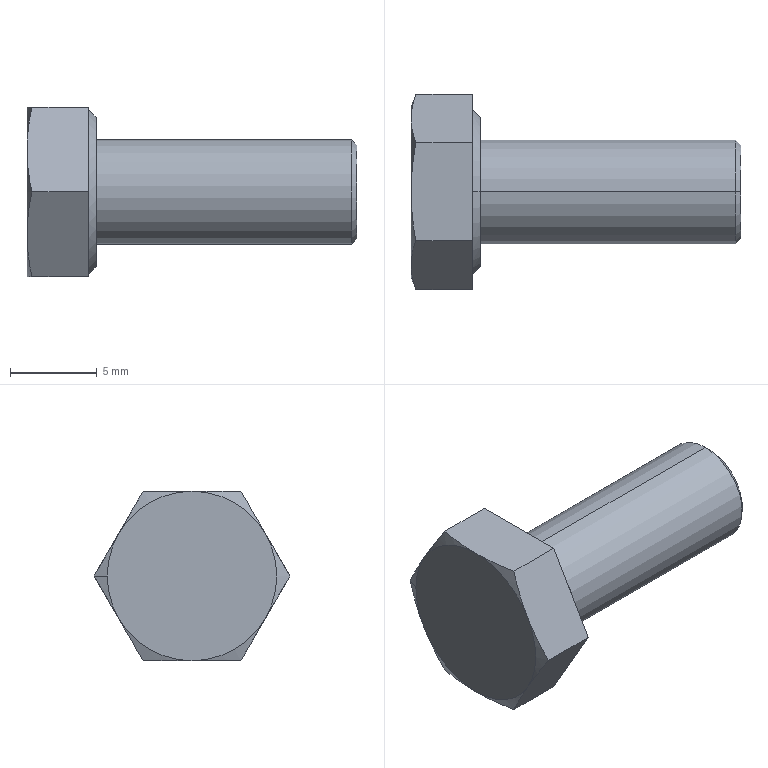Part | SolidWorks | features BaseBody 1, MoveFace 1, Scale 1 | 1 solid | 23 faces | box 18.975 x 11.258 x 9.75 mm | volume 741.836 mm3 | cone 11 | plane 10 | cylinder 2 | commonest cylinder face diameters 6 x2
STEP:
#1=CARTESIAN_POINT('',(18.675,0.,3.));
#2=VERTEX_POINT('',#1);
#3=CARTESIAN_POINT('',(18.675,0.,-3.));
#4=VERTEX_POINT('',#3);
#5=CARTESIAN_POINT('',(18.675,0.,0.));
#6=DIRECTION('',(-1.,0.,0.));
#7=DIRECTION('',(0.,0.,1.));
#8=AXIS2_PLACEMENT_3D('',#5,#6,#7);
#9=CIRCLE('',#8,3.);
#10=EDGE_CURVE('',#2,#4,#9,.T.);
#11=ORIENTED_EDGE('',*,*,#10,.T.);
#12=CARTESIAN_POINT('',(3.975,0.,-3.));
#13=VERTEX_POINT('',#12);
#14=CARTESIAN_POINT('',(33.975,0.,-3.));
#15=DIRECTION('',(-1.,0.,0.));
#16=VECTOR('',#15,1000.);
#17=LINE('',#14,#16);
#18=EDGE_CURVE('',#4,#13,#17,.T.);
#19=ORIENTED_EDGE('',*,*,#18,.T.);
#20=CARTESIAN_POINT('',(3.975,0.,3.));
#21=VERTEX_POINT('',#20);
#22=CARTESIAN_POINT('',(3.975,0.,0.));
#23=DIRECTION('',(1.,0.,0.));
#24=DIRECTION('',(0.,0.,1.));
#25=AXIS2_PLACEMENT_3D('',#22,#23,#24);
#26=CIRCLE('',#25,3.);
#27=EDGE_CURVE('',#13,#21,#26,.T.);
#28=ORIENTED_EDGE('',*,*,#27,.T.);
#29=CARTESIAN_POINT('',(33.975,0.,3.));
#30=DIRECTION('',(-1.,0.,0.));
#31=VECTOR('',#30,1000.);
#32=LINE('',#29,#31);
#33=EDGE_CURVE('',#2,#21,#32,.T.);
#34=ORIENTED_EDGE('',*,*,#33,.F.);
#35=EDGE_LOOP('',(#11,#19,#28,#34));
#36=FACE_OUTER_BOUND('',#35,.T.);
#37=CARTESIAN_POINT('',(33.975,0.,0.));
#38=DIRECTION('',(-1.,0.,0.));
#39=DIRECTION('',(0.,0.,1.));
#40=AXIS2_PLACEMENT_3D('',#37,#38,#39);
#41=CYLINDRICAL_SURFACE('',#40,3.);
#42=ADVANCED_FACE('',(#36),#41,.T.);
#43=CARTESIAN_POINT('',(18.975,0.,2.7));
#44=VERTEX_POINT('',#43);
#45=CARTESIAN_POINT('',(18.975,0.,-2.7));
#46=VERTEX_POINT('',#45);
#47=CARTESIAN_POINT('',(18.975,0.,0.));
#48=DIRECTION('',(-1.,0.,0.));
#49=DIRECTION('',(0.,0.,1.));
#50=AXIS2_PLACEMENT_3D('',#47,#48,#49);
#51=CIRCLE('',#50,2.7);
#52=EDGE_CURVE('',#44,#46,#51,.T.);
#53=ORIENTED_EDGE('',*,*,#52,.T.);
#54=CARTESIAN_POINT('',(18.675,0.,-3.));
#55=DIRECTION('',(-0.7071,0.,-0.7071));
#56=VECTOR('',#55,1000.);
#57=LINE('',#54,#56);
#58=EDGE_CURVE('',#46,#4,#57,.T.);
#59=ORIENTED_EDGE('',*,*,#58,.T.);
#60=ORIENTED_EDGE('',*,*,#10,.F.);
#61=CARTESIAN_POINT('',(18.675,0.,3.));
#62=DIRECTION('',(-0.7071,0.,0.7071));
#63=VECTOR('',#62,1000.);
#64=LINE('',#61,#63);
#65=EDGE_CURVE('',#44,#2,#64,.T.);
#66=ORIENTED_EDGE('',*,*,#65,.F.);
#67=EDGE_LOOP('',(#53,#59,#60,#66));
#68=FACE_OUTER_BOUND('',#67,.T.);
#69=CARTESIAN_POINT('',(18.675,0.,0.));
#70=DIRECTION('',(-1.,0.,0.));
#71=DIRECTION('',(0.,0.,1.));
#72=AXIS2_PLACEMENT_3D('',#69,#70,#71);
#73=CONICAL_SURFACE('',#72,3.,0.7854);
#74=ADVANCED_FACE('',(#68),#73,.T.);
#75=CARTESIAN_POINT('',(3.975,0.,4.301));
#76=VERTEX_POINT('',#75);
#77=CARTESIAN_POINT('',(3.975,0.,-4.301));
#78=VERTEX_POINT('',#77);
#79=CARTESIAN_POINT('',(3.975,0.,0.));
#80=DIRECTION('',(-1.,0.,0.));
#81=DIRECTION('',(0.,0.,1.));
#82=AXIS2_PLACEMENT_3D('',#79,#80,#81);
#83=CIRCLE('',#82,4.301);
#84=EDGE_CURVE('',#76,#78,#83,.T.);
#85=ORIENTED_EDGE('',*,*,#84,.T.);
#86=CARTESIAN_POINT('',(3.525,0.,-4.751));
#87=VERTEX_POINT('',#86);
#88=CARTESIAN_POINT('',(3.525,0.,-4.751));
#89=DIRECTION('',(-0.7071,0.,-0.7071));
#90=VECTOR('',#89,1000.);
#91=LINE('',#88,#90);
#92=EDGE_CURVE('',#78,#87,#91,.T.);
#93=ORIENTED_EDGE('',*,*,#92,.T.);
#94=CARTESIAN_POINT('',(3.525,0.,4.751));
#95=VERTEX_POINT('',#94);
#96=CARTESIAN_POINT('',(3.525,0.,0.));
#97=DIRECTION('',(1.,0.,0.));
#98=DIRECTION('',(0.,0.,1.));
#99=AXIS2_PLACEMENT_3D('',#96,#97,#98);
#100=CIRCLE('',#99,4.751);
#101=EDGE_CURVE('',#87,#95,#100,.T.);
#102=ORIENTED_EDGE('',*,*,#101,.T.);
#103=CARTESIAN_POINT('',(3.525,0.,4.751));
#104=DIRECTION('',(-0.7071,0.,0.7071));
#105=VECTOR('',#104,1000.);
#106=LINE('',#103,#105);
#107=EDGE_CURVE('',#76,#95,#106,.T.);
#108=ORIENTED_EDGE('',*,*,#107,.F.);
#109=EDGE_LOOP('',(#85,#93,#102,#108));
#110=FACE_OUTER_BOUND('',#109,.T.);
#111=CARTESIAN_POINT('',(3.525,0.,0.));
#112=DIRECTION('',(-1.,0.,0.));
#113=DIRECTION('',(0.,0.,1.));
#114=AXIS2_PLACEMENT_3D('',#111,#112,#113);
#115=CONICAL_SURFACE('',#114,4.751,0.7854);
#116=ADVANCED_FACE('',(#110),#115,.T.);
#117=CARTESIAN_POINT('',(0.,4.222,-2.437));
#118=VERTEX_POINT('',#117);
#119=CARTESIAN_POINT('',(0.,4.875,0.));
#120=VERTEX_POINT('',#119);
#121=CARTESIAN_POINT('',(0.,0.,0.));
#122=DIRECTION('',(1.,0.,0.));
#123=DIRECTION('',(0.,1.,0.));
#124=AXIS2_PLACEMENT_3D('',#121,#122,#123);
#125=CIRCLE('',#124,4.875);
#126=EDGE_CURVE('',#118,#120,#125,.T.);
#127=ORIENTED_EDGE('',*,*,#126,.T.);
#128=CARTESIAN_POINT('',(0.2745,5.629,0.));
#129=VERTEX_POINT('',#128);
#130=CARTESIAN_POINT('',(0.2761,5.634,0.));
#131=DIRECTION('',(0.342,0.9397,0.));
#132=VECTOR('',#131,1000.);
#133=LINE('',#130,#132);
#134=EDGE_CURVE('',#120,#129,#133,.T.);
#135=ORIENTED_EDGE('',*,*,#134,.T.);
#136=CARTESIAN_POINT('',(0.2745,5.629,0.));
#137=CARTESIAN_POINT('',(0.1051,5.164,-0.8059));
#138=CARTESIAN_POINT('',(0.,4.695,-1.617));
#139=CARTESIAN_POINT('',(0.,4.222,-2.437));
#140=B_SPLINE_CURVE_WITH_KNOTS('',3,(#136,#137,#138,#139),.UNSPECIFIED.,.F.,.F.,(4,4),(0.,0.002828),.UNSPECIFIED.);
#141=EDGE_CURVE('',#129,#118,#140,.T.);
#142=ORIENTED_EDGE('',*,*,#141,.T.);
#143=EDGE_LOOP('',(#127,#135,#142));
#144=FACE_OUTER_BOUND('',#143,.T.);
#145=CARTESIAN_POINT('',(0.2761,0.,0.));
#146=DIRECTION('',(1.,0.,0.));
#147=DIRECTION('',(0.,1.,0.));
#148=AXIS2_PLACEMENT_3D('',#145,#146,#147);
#149=CONICAL_SURFACE('',#148,5.634,1.222);
#150=ADVANCED_FACE('',(#144),#149,.T.);
#151=ORIENTED_EDGE('',*,*,#18,.F.);
#152=CARTESIAN_POINT('',(18.675,0.,0.));
#153=DIRECTION('',(-1.,0.,0.));
#154=DIRECTION('',(0.,0.,1.));
#155=AXIS2_PLACEMENT_3D('',#152,#153,#154);
#156=CIRCLE('',#155,3.);
#157=EDGE_CURVE('',#4,#2,#156,.T.);
#158=ORIENTED_EDGE('',*,*,#157,.T.);
#159=ORIENTED_EDGE('',*,*,#33,.T.);
#160=CARTESIAN_POINT('',(3.975,0.,0.));
#161=DIRECTION('',(1.,0.,0.));
#162=DIRECTION('',(0.,0.,1.));
#163=AXIS2_PLACEMENT_3D('',#160,#161,#162);
#164=CIRCLE('',#163,3.);
#165=EDGE_CURVE('',#21,#13,#164,.T.);
#166=ORIENTED_EDGE('',*,*,#165,.T.);
#167=EDGE_LOOP('',(#151,#158,#159,#166));
#168=FACE_OUTER_BOUND('',#167,.T.);
#169=CARTESIAN_POINT('',(33.975,0.,0.));
#170=DIRECTION('',(-1.,0.,0.));
#171=DIRECTION('',(0.,0.,1.));
#172=AXIS2_PLACEMENT_3D('',#169,#170,#171);
#173=CYLINDRICAL_SURFACE('',#172,3.);
#174=ADVANCED_FACE('',(#168),#173,.T.);
#175=ORIENTED_EDGE('',*,*,#165,.F.);
#176=ORIENTED_EDGE('',*,*,#27,.F.);
#177=EDGE_LOOP('',(#175,#176));
#178=FACE_BOUND('',#177,.T.);
#179=ORIENTED_EDGE('',*,*,#84,.F.);
#180=CARTESIAN_POINT('',(3.975,0.,0.));
#181=DIRECTION('',(-1.,0.,0.));
#182=DIRECTION('',(0.,0.,1.));
#183=AXIS2_PLACEMENT_3D('',#180,#181,#182);
#184=CIRCLE('',#183,4.301);
#185=EDGE_CURVE('',#78,#76,#184,.T.);
#186=ORIENTED_EDGE('',*,*,#185,.F.);
#187=EDGE_LOOP('',(#179,#186));
#188=FACE_OUTER_BOUND('',#187,.T.);
#189=CARTESIAN_POINT('',(3.975,0.,9.75));
#190=DIRECTION('',(-1.,0.,0.));
#191=DIRECTION('',(0.,0.,1.));
#192=AXIS2_PLACEMENT_3D('',#189,#190,#191);
#193=PLANE('',#192);
#194=ADVANCED_FACE('',(#178,#188),#193,.F.);
#195=ORIENTED_EDGE('',*,*,#58,.F.);
#196=CARTESIAN_POINT('',(18.975,0.,0.));
#197=DIRECTION('',(-1.,0.,0.));
#198=DIRECTION('',(0.,0.,1.));
#199=AXIS2_PLACEMENT_3D('',#196,#197,#198);
#200=CIRCLE('',#199,2.7);
#201=EDGE_CURVE('',#46,#44,#200,.T.);
#202=ORIENTED_EDGE('',*,*,#201,.T.);
#203=ORIENTED_EDGE('',*,*,#65,.T.);
#204=ORIENTED_EDGE('',*,*,#157,.F.);
#205=EDGE_LOOP('',(#195,#202,#203,#204));
#206=FACE_OUTER_BOUND('',#205,.T.);
#207=CARTESIAN_POINT('',(18.675,0.,0.));
#208=DIRECTION('',(-1.,0.,0.));
#209=DIRECTION('',(0.,0.,1.));
#210=AXIS2_PLACEMENT_3D('',#207,#208,#209);
#211=CONICAL_SURFACE('',#210,3.,0.7854);
#212=ADVANCED_FACE('',(#206),#211,.T.);
#213=ORIENTED_EDGE('',*,*,#92,.F.);
#214=ORIENTED_EDGE('',*,*,#185,.T.);
#215=ORIENTED_EDGE('',*,*,#107,.T.);
#216=CARTESIAN_POINT('',(3.525,0.,0.));
#217=DIRECTION('',(1.,0.,0.));
#218=DIRECTION('',(0.,0.,1.));
#219=AXIS2_PLACEMENT_3D('',#216,#217,#218);
#220=CIRCLE('',#219,4.751);
#221=EDGE_CURVE('',#95,#87,#220,.T.);
#222=ORIENTED_EDGE('',*,*,#221,.T.);
#223=EDGE_LOOP('',(#213,#214,#215,#222));
#224=FACE_OUTER_BOUND('',#223,.T.);
#225=CARTESIAN_POINT('',(3.525,0.,0.));
#226=DIRECTION('',(-1.,0.,0.));
#227=DIRECTION('',(0.,0.,1.));
#228=AXIS2_PLACEMENT_3D('',#225,#226,#227);
#229=CONICAL_SURFACE('',#228,4.751,0.7854);
#230=ADVANCED_FACE('',(#224),#229,.T.);
#231=ORIENTED_EDGE('',*,*,#52,.F.);
#232=ORIENTED_EDGE('',*,*,#201,.F.);
#233=EDGE_LOOP('',(#231,#232));
#234=FACE_OUTER_BOUND('',#233,.T.);
#235=CARTESIAN_POINT('',(18.975,0.,0.));
#236=DIRECTION('',(1.,0.,0.));
#237=DIRECTION('',(0.,0.,-1.));
#238=AXIS2_PLACEMENT_3D('',#235,#236,#237);
#239=PLANE('',#238);
#240=ADVANCED_FACE('',(#234),#239,.T.);
#241=CARTESIAN_POINT('',(3.525,5.629,0.));
#242=VERTEX_POINT('',#241);
#243=CARTESIAN_POINT('',(3.525,2.815,4.875));
#244=VERTEX_POINT('',#243);
#245=CARTESIAN_POINT('',(3.525,5.629,0.));
#246=DIRECTION('',(0.,-0.5,0.866));
#247=VECTOR('',#246,1000.);
#248=LINE('',#245,#247);
#249=EDGE_CURVE('',#242,#244,#248,.T.);
#250=ORIENTED_EDGE('',*,*,#249,.T.);
#251=CARTESIAN_POINT('',(3.525,-2.815,4.875));
#252=VERTEX_POINT('',#251);
#253=CARTESIAN_POINT('',(3.525,4.751,4.875));
#254=DIRECTION('',(0.,-1.,0.));
#255=VECTOR('',#254,1000.);
#256=LINE('',#253,#255);
#257=EDGE_CURVE('',#244,#252,#256,.T.);
#258=ORIENTED_EDGE('',*,*,#257,.T.);
#259=CARTESIAN_POINT('',(3.525,-5.629,0.));
#260=VERTEX_POINT('',#259);
#261=CARTESIAN_POINT('',(3.525,-2.815,4.875));
#262=DIRECTION('',(0.,-0.5,-0.866));
#263=VECTOR('',#262,1000.);
#264=LINE('',#261,#263);
#265=EDGE_CURVE('',#252,#260,#264,.T.);
#266=ORIENTED_EDGE('',*,*,#265,.T.);
#267=CARTESIAN_POINT('',(3.525,-2.815,-4.875));
#268=VERTEX_POINT('',#267);
#269=CARTESIAN_POINT('',(3.525,-5.629,0.));
#270=DIRECTION('',(0.,0.5,-0.866));
#271=VECTOR('',#270,1000.);
#272=LINE('',#269,#271);
#273=EDGE_CURVE('',#260,#268,#272,.T.);
#274=ORIENTED_EDGE('',*,*,#273,.T.);
#275=CARTESIAN_POINT('',(3.525,2.815,-4.875));
#276=VERTEX_POINT('',#275);
#277=CARTESIAN_POINT('',(3.525,4.751,-4.875));
#278=DIRECTION('',(0.,1.,0.));
#279=VECTOR('',#278,1000.);
#280=LINE('',#277,#279);
#281=EDGE_CURVE('',#268,#276,#280,.T.);
#282=ORIENTED_EDGE('',*,*,#281,.T.);
#283=CARTESIAN_POINT('',(3.525,2.815,-4.875));
#284=DIRECTION('',(0.,0.5,0.866));
#285=VECTOR('',#284,1000.);
#286=LINE('',#283,#285);
#287=EDGE_CURVE('',#276,#242,#286,.T.);
#288=ORIENTED_EDGE('',*,*,#287,.T.);
#289=EDGE_LOOP('',(#250,#258,#266,#274,#282,#288));
#290=FACE_OUTER_BOUND('',#289,.T.);
#291=ORIENTED_EDGE('',*,*,#221,.F.);
#292=ORIENTED_EDGE('',*,*,#101,.F.);
#293=EDGE_LOOP('',(#291,#292));
#294=FACE_BOUND('',#293,.T.);
#295=CARTESIAN_POINT('',(3.525,4.751,0.));
#296=DIRECTION('',(1.,0.,0.));
#297=DIRECTION('',(0.,0.,-1.));
#298=AXIS2_PLACEMENT_3D('',#295,#296,#297);
#299=PLANE('',#298);
#300=ADVANCED_FACE('',(#290,#294),#299,.T.);
#301=CARTESIAN_POINT('',(0.2745,-2.815,4.875));
#302=VERTEX_POINT('',#301);
#303=CARTESIAN_POINT('',(3.975,-2.815,4.875));
#304=DIRECTION('',(-1.,0.,0.));
#305=VECTOR('',#304,1000.);
#306=LINE('',#303,#305);
#307=EDGE_CURVE('',#252,#302,#306,.T.);
#308=ORIENTED_EDGE('',*,*,#307,.F.);
#309=ORIENTED_EDGE('',*,*,#257,.F.);
#310=CARTESIAN_POINT('',(0.2745,2.815,4.875));
#311=VERTEX_POINT('',#310);
#312=CARTESIAN_POINT('',(3.975,2.815,4.875));
#313=DIRECTION('',(1.,0.,0.));
#314=VECTOR('',#313,1000.);
#315=LINE('',#312,#314);
#316=EDGE_CURVE('',#311,#244,#315,.T.);
#317=ORIENTED_EDGE('',*,*,#316,.F.);
#318=CARTESIAN_POINT('',(0.,0.,4.875));
#319=VERTEX_POINT('',#318);
#320=CARTESIAN_POINT('',(0.,0.,4.875));
#321=CARTESIAN_POINT('',(0.,0.9471,4.875));
#322=CARTESIAN_POINT('',(0.1051,1.884,4.875));
#323=CARTESIAN_POINT('',(0.2745,2.815,4.875));
#324=B_SPLINE_CURVE_WITH_KNOTS('',3,(#320,#321,#322,#323),.UNSPECIFIED.,.F.,.F.,(4,4),(0.,0.002828),.UNSPECIFIED.);
#325=EDGE_CURVE('',#319,#311,#324,.T.);
#326=ORIENTED_EDGE('',*,*,#325,.F.);
#327=CARTESIAN_POINT('',(0.2745,-2.815,4.875));
#328=CARTESIAN_POINT('',(0.1051,-1.884,4.875));
#329=CARTESIAN_POINT('',(0.,-0.9471,4.875));
#330=CARTESIAN_POINT('',(0.,0.,4.875));
#331=B_SPLINE_CURVE_WITH_KNOTS('',3,(#327,#328,#329,#330),.UNSPECIFIED.,.F.,.F.,(4,4),(0.,0.002828),.UNSPECIFIED.);
#332=EDGE_CURVE('',#302,#319,#331,.T.);
#333=ORIENTED_EDGE('',*,*,#332,.F.);
#334=EDGE_LOOP('',(#308,#309,#317,#326,#333));
#335=FACE_OUTER_BOUND('',#334,.T.);
#336=CARTESIAN_POINT('',(3.975,2.815,4.875));
#337=DIRECTION('',(0.,0.,-1.));
#338=DIRECTION('',(-1.,0.,0.));
#339=AXIS2_PLACEMENT_3D('',#336,#337,#338);
#340=PLANE('',#339);
#341=ADVANCED_FACE('',(#335),#340,.F.);
#342=ORIENTED_EDGE('',*,*,#316,.T.);
#343=ORIENTED_EDGE('',*,*,#249,.F.);
#344=CARTESIAN_POINT('',(3.975,5.629,0.));
#345=DIRECTION('',(1.,0.,0.));
#346=VECTOR('',#345,1000.);
#347=LINE('',#344,#346);
#348=EDGE_CURVE('',#129,#242,#347,.T.);
#349=ORIENTED_EDGE('',*,*,#348,.F.);
#350=CARTESIAN_POINT('',(0.,4.222,2.437));
#351=VERTEX_POINT('',#350);
#352=CARTESIAN_POINT('',(0.,4.222,2.437));
#353=CARTESIAN_POINT('',(0.,4.695,1.617));
#354=CARTESIAN_POINT('',(0.1051,5.164,0.8059));
#355=CARTESIAN_POINT('',(0.2745,5.629,0.));
#356=B_SPLINE_CURVE_WITH_KNOTS('',3,(#352,#353,#354,#355),.UNSPECIFIED.,.F.,.F.,(4,4),(0.,0.002828),.UNSPECIFIED.);
#357=EDGE_CURVE('',#351,#129,#356,.T.);
#358=ORIENTED_EDGE('',*,*,#357,.F.);
#359=CARTESIAN_POINT('',(0.2745,2.815,4.875));
#360=CARTESIAN_POINT('',(0.1051,3.28,4.069));
#361=CARTESIAN_POINT('',(0.,3.748,3.258));
#362=CARTESIAN_POINT('',(0.,4.222,2.437));
#363=B_SPLINE_CURVE_WITH_KNOTS('',3,(#359,#360,#361,#362),.UNSPECIFIED.,.F.,.F.,(4,4),(0.,0.002828),.UNSPECIFIED.);
#364=EDGE_CURVE('',#311,#351,#363,.T.);
#365=ORIENTED_EDGE('',*,*,#364,.F.);
#366=EDGE_LOOP('',(#342,#343,#349,#358,#365));
#367=FACE_OUTER_BOUND('',#366,.T.);
#368=CARTESIAN_POINT('',(3.975,5.629,0.));
#369=DIRECTION('',(0.,-0.866,-0.5));
#370=DIRECTION('',(0.,0.5,-0.866));
#371=AXIS2_PLACEMENT_3D('',#368,#369,#370);
#372=PLANE('',#371);
#373=ADVANCED_FACE('',(#367),#372,.F.);
#374=ORIENTED_EDGE('',*,*,#348,.T.);
#375=ORIENTED_EDGE('',*,*,#287,.F.);
#376=CARTESIAN_POINT('',(0.2745,2.815,-4.875));
#377=VERTEX_POINT('',#376);
#378=CARTESIAN_POINT('',(3.975,2.815,-4.875));
#379=DIRECTION('',(1.,0.,0.));
#380=VECTOR('',#379,1000.);
#381=LINE('',#378,#380);
#382=EDGE_CURVE('',#377,#276,#381,.T.);
#383=ORIENTED_EDGE('',*,*,#382,.F.);
#384=CARTESIAN_POINT('',(0.,4.222,-2.437));
#385=CARTESIAN_POINT('',(0.,3.748,-3.258));
#386=CARTESIAN_POINT('',(0.1051,3.28,-4.069));
#387=CARTESIAN_POINT('',(0.2745,2.815,-4.875));
#388=B_SPLINE_CURVE_WITH_KNOTS('',3,(#384,#385,#386,#387),.UNSPECIFIED.,.F.,.F.,(4,4),(0.,0.002828),.UNSPECIFIED.);
#389=EDGE_CURVE('',#118,#377,#388,.T.);
#390=ORIENTED_EDGE('',*,*,#389,.F.);
#391=ORIENTED_EDGE('',*,*,#141,.F.);
#392=EDGE_LOOP('',(#374,#375,#383,#390,#391));
#393=FACE_OUTER_BOUND('',#392,.T.);
#394=CARTESIAN_POINT('',(3.975,2.815,-4.875));
#395=DIRECTION('',(0.,-0.866,0.5));
#396=DIRECTION('',(0.,-0.5,-0.866));
#397=AXIS2_PLACEMENT_3D('',#394,#395,#396);
#398=PLANE('',#397);
#399=ADVANCED_FACE('',(#393),#398,.F.);
#400=ORIENTED_EDGE('',*,*,#382,.T.);
#401=ORIENTED_EDGE('',*,*,#281,.F.);
#402=CARTESIAN_POINT('',(0.2745,-2.815,-4.875));
#403=VERTEX_POINT('',#402);
#404=CARTESIAN_POINT('',(3.975,-2.815,-4.875));
#405=DIRECTION('',(1.,0.,0.));
#406=VECTOR('',#405,1000.);
#407=LINE('',#404,#406);
#408=EDGE_CURVE('',#403,#268,#407,.T.);
#409=ORIENTED_EDGE('',*,*,#408,.F.);
#410=CARTESIAN_POINT('',(0.,0.,-4.875));
#411=VERTEX_POINT('',#410);
#412=CARTESIAN_POINT('',(0.,0.,-4.875));
#413=CARTESIAN_POINT('',(0.,-0.9471,-4.875));
#414=CARTESIAN_POINT('',(0.1051,-1.884,-4.875));
#415=CARTESIAN_POINT('',(0.2745,-2.815,-4.875));
#416=B_SPLINE_CURVE_WITH_KNOTS('',3,(#412,#413,#414,#415),.UNSPECIFIED.,.F.,.F.,(4,4),(0.,0.002828),.UNSPECIFIED.);
#417=EDGE_CURVE('',#411,#403,#416,.T.);
#418=ORIENTED_EDGE('',*,*,#417,.F.);
#419=CARTESIAN_POINT('',(0.2745,2.815,-4.875));
#420=CARTESIAN_POINT('',(0.1051,1.884,-4.875));
#421=CARTESIAN_POINT('',(0.,0.9471,-4.875));
#422=CARTESIAN_POINT('',(0.,0.,-4.875));
#423=B_SPLINE_CURVE_WITH_KNOTS('',3,(#419,#420,#421,#422),.UNSPECIFIED.,.F.,.F.,(4,4),(0.,0.002828),.UNSPECIFIED.);
#424=EDGE_CURVE('',#377,#411,#423,.T.);
#425=ORIENTED_EDGE('',*,*,#424,.F.);
#426=EDGE_LOOP('',(#400,#401,#409,#418,#425));
#427=FACE_OUTER_BOUND('',#426,.T.);
#428=CARTESIAN_POINT('',(3.975,-2.815,-4.875));
#429=DIRECTION('',(0.,0.,1.));
#430=DIRECTION('',(1.,0.,0.));
#431=AXIS2_PLACEMENT_3D('',#428,#429,#430);
#432=PLANE('',#431);
#433=ADVANCED_FACE('',(#427),#432,.F.);
#434=ORIENTED_EDGE('',*,*,#408,.T.);
#435=ORIENTED_EDGE('',*,*,#273,.F.);
#436=CARTESIAN_POINT('',(0.2745,-5.629,0.));
#437=VERTEX_POINT('',#436);
#438=CARTESIAN_POINT('',(3.975,-5.629,0.));
#439=DIRECTION('',(1.,0.,0.));
#440=VECTOR('',#439,1000.);
#441=LINE('',#438,#440);
#442=EDGE_CURVE('',#437,#260,#441,.T.);
#443=ORIENTED_EDGE('',*,*,#442,.F.);
#444=CARTESIAN_POINT('',(0.,-4.222,-2.437));
#445=VERTEX_POINT('',#444);
#446=CARTESIAN_POINT('',(0.,-4.222,-2.437));
#447=CARTESIAN_POINT('',(0.,-4.695,-1.617));
#448=CARTESIAN_POINT('',(0.1051,-5.164,-0.8059));
#449=CARTESIAN_POINT('',(0.2745,-5.629,0.));
#450=B_SPLINE_CURVE_WITH_KNOTS('',3,(#446,#447,#448,#449),.UNSPECIFIED.,.F.,.F.,(4,4),(0.,0.002828),.UNSPECIFIED.);
#451=EDGE_CURVE('',#445,#437,#450,.T.);
#452=ORIENTED_EDGE('',*,*,#451,.F.);
#453=CARTESIAN_POINT('',(0.2745,-2.815,-4.875));
#454=CARTESIAN_POINT('',(0.1051,-3.28,-4.069));
#455=CARTESIAN_POINT('',(0.,-3.748,-3.258));
#456=CARTESIAN_POINT('',(0.,-4.222,-2.437));
#457=B_SPLINE_CURVE_WITH_KNOTS('',3,(#453,#454,#455,#456),.UNSPECIFIED.,.F.,.F.,(4,4),(0.,0.002828),.UNSPECIFIED.);
#458=EDGE_CURVE('',#403,#445,#457,.T.);
#459=ORIENTED_EDGE('',*,*,#458,.F.);
#460=EDGE_LOOP('',(#434,#435,#443,#452,#459));
#461=FACE_OUTER_BOUND('',#460,.T.);
#462=CARTESIAN_POINT('',(3.975,-5.629,0.));
#463=DIRECTION('',(0.,0.866,0.5));
#464=DIRECTION('',(0.,-0.5,0.866));
#465=AXIS2_PLACEMENT_3D('',#462,#463,#464);
#466=PLANE('',#465);
#467=ADVANCED_FACE('',(#461),#466,.F.);
#468=ORIENTED_EDGE('',*,*,#442,.T.);
#469=ORIENTED_EDGE('',*,*,#265,.F.);
#470=ORIENTED_EDGE('',*,*,#307,.T.);
#471=CARTESIAN_POINT('',(0.,-4.222,2.437));
#472=VERTEX_POINT('',#471);
#473=CARTESIAN_POINT('',(0.,-4.222,2.437));
#474=CARTESIAN_POINT('',(0.,-3.748,3.258));
#475=CARTESIAN_POINT('',(0.1051,-3.28,4.069));
#476=CARTESIAN_POINT('',(0.2745,-2.815,4.875));
#477=B_SPLINE_CURVE_WITH_KNOTS('',3,(#473,#474,#475,#476),.UNSPECIFIED.,.F.,.F.,(4,4),(0.,0.002828),.UNSPECIFIED.);
#478=EDGE_CURVE('',#472,#302,#477,.T.);
#479=ORIENTED_EDGE('',*,*,#478,.F.);
#480=CARTESIAN_POINT('',(0.2745,-5.629,0.));
#481=CARTESIAN_POINT('',(0.1051,-5.164,0.8059));
#482=CARTESIAN_POINT('',(0.,-4.695,1.617));
#483=CARTESIAN_POINT('',(0.,-4.222,2.437));
#484=B_SPLINE_CURVE_WITH_KNOTS('',3,(#480,#481,#482,#483),.UNSPECIFIED.,.F.,.F.,(4,4),(0.,0.002828),.UNSPECIFIED.);
#485=EDGE_CURVE('',#437,#472,#484,.T.);
#486=ORIENTED_EDGE('',*,*,#485,.F.);
#487=EDGE_LOOP('',(#468,#469,#470,#479,#486));
#488=FACE_OUTER_BOUND('',#487,.T.);
#489=CARTESIAN_POINT('',(3.975,-2.815,4.875));
#490=DIRECTION('',(0.,0.866,-0.5));
#491=DIRECTION('',(0.,0.5,0.866));
#492=AXIS2_PLACEMENT_3D('',#489,#490,#491);
#493=PLANE('',#492);
#494=ADVANCED_FACE('',(#488),#493,.F.);
#495=ORIENTED_EDGE('',*,*,#332,.T.);
#496=CARTESIAN_POINT('',(0.,0.,0.));
#497=DIRECTION('',(1.,0.,0.));
#498=DIRECTION('',(0.,1.,0.));
#499=AXIS2_PLACEMENT_3D('',#496,#497,#498);
#500=CIRCLE('',#499,4.875);
#501=EDGE_CURVE('',#319,#472,#500,.T.);
#502=ORIENTED_EDGE('',*,*,#501,.T.);
#503=ORIENTED_EDGE('',*,*,#478,.T.);
#504=EDGE_LOOP('',(#495,#502,#503));
#505=FACE_OUTER_BOUND('',#504,.T.);
#506=CARTESIAN_POINT('',(0.2761,0.,0.));
#507=DIRECTION('',(1.,0.,0.));
#508=DIRECTION('',(0.,1.,0.));
#509=AXIS2_PLACEMENT_3D('',#506,#507,#508);
#510=CONICAL_SURFACE('',#509,5.634,1.222);
#511=ADVANCED_FACE('',(#505),#510,.T.);
#512=CARTESIAN_POINT('',(0.,0.,0.));
#513=DIRECTION('',(1.,0.,0.));
#514=DIRECTION('',(0.,1.,0.));
#515=AXIS2_PLACEMENT_3D('',#512,#513,#514);
#516=CIRCLE('',#515,4.875);
#517=EDGE_CURVE('',#351,#319,#516,.T.);
#518=ORIENTED_EDGE('',*,*,#517,.T.);
#519=ORIENTED_EDGE('',*,*,#325,.T.);
#520=ORIENTED_EDGE('',*,*,#364,.T.);
#521=EDGE_LOOP('',(#518,#519,#520));
#522=FACE_OUTER_BOUND('',#521,.T.);
#523=CARTESIAN_POINT('',(0.2761,0.,0.));
#524=DIRECTION('',(1.,0.,0.));
#525=DIRECTION('',(0.,1.,0.));
#526=AXIS2_PLACEMENT_3D('',#523,#524,#525);
#527=CONICAL_SURFACE('',#526,5.634,1.222);
#528=ADVANCED_FACE('',(#522),#527,.T.);
#529=ORIENTED_EDGE('',*,*,#134,.F.);
#530=CARTESIAN_POINT('',(0.,0.,0.));
#531=DIRECTION('',(1.,0.,0.));
#532=DIRECTION('',(0.,1.,0.));
#533=AXIS2_PLACEMENT_3D('',#530,#531,#532);
#534=CIRCLE('',#533,4.875);
#535=EDGE_CURVE('',#120,#351,#534,.T.);
#536=ORIENTED_EDGE('',*,*,#535,.T.);
#537=ORIENTED_EDGE('',*,*,#357,.T.);
#538=EDGE_LOOP('',(#529,#536,#537));
#539=FACE_OUTER_BOUND('',#538,.T.);
#540=CARTESIAN_POINT('',(0.2761,0.,0.));
#541=DIRECTION('',(1.,0.,0.));
#542=DIRECTION('',(0.,1.,0.));
#543=AXIS2_PLACEMENT_3D('',#540,#541,#542);
#544=CONICAL_SURFACE('',#543,5.634,1.222);
#545=ADVANCED_FACE('',(#539),#544,.T.);
#546=CARTESIAN_POINT('',(0.,0.,0.));
#547=DIRECTION('',(1.,0.,0.));
#548=DIRECTION('',(0.,1.,0.));
#549=AXIS2_PLACEMENT_3D('',#546,#547,#548);
#550=CIRCLE('',#549,4.875);
#551=EDGE_CURVE('',#411,#118,#550,.T.);
#552=ORIENTED_EDGE('',*,*,#551,.T.);
#553=ORIENTED_EDGE('',*,*,#389,.T.);
#554=ORIENTED_EDGE('',*,*,#424,.T.);
#555=EDGE_LOOP('',(#552,#553,#554));
#556=FACE_OUTER_BOUND('',#555,.T.);
#557=CARTESIAN_POINT('',(0.2761,0.,0.));
#558=DIRECTION('',(1.,0.,0.));
#559=DIRECTION('',(0.,1.,0.));
#560=AXIS2_PLACEMENT_3D('',#557,#558,#559);
#561=CONICAL_SURFACE('',#560,5.634,1.222);
#562=ADVANCED_FACE('',(#556),#561,.T.);
#563=ORIENTED_EDGE('',*,*,#458,.T.);
#564=CARTESIAN_POINT('',(0.,0.,0.));
#565=DIRECTION('',(1.,0.,0.));
#566=DIRECTION('',(0.,1.,0.));
#567=AXIS2_PLACEMENT_3D('',#564,#565,#566);
#568=CIRCLE('',#567,4.875);
#569=EDGE_CURVE('',#445,#411,#568,.T.);
#570=ORIENTED_EDGE('',*,*,#569,.T.);
#571=ORIENTED_EDGE('',*,*,#417,.T.);
#572=EDGE_LOOP('',(#563,#570,#571));
#573=FACE_OUTER_BOUND('',#572,.T.);
#574=CARTESIAN_POINT('',(0.2761,0.,0.));
#575=DIRECTION('',(1.,0.,0.));
#576=DIRECTION('',(0.,1.,0.));
#577=AXIS2_PLACEMENT_3D('',#574,#575,#576);
#578=CONICAL_SURFACE('',#577,5.634,1.222);
#579=ADVANCED_FACE('',(#573),#578,.T.);
#580=ORIENTED_EDGE('',*,*,#485,.T.);
#581=CARTESIAN_POINT('',(0.,0.,0.));
#582=DIRECTION('',(1.,0.,0.));
#583=DIRECTION('',(0.,1.,0.));
#584=AXIS2_PLACEMENT_3D('',#581,#582,#583);
#585=CIRCLE('',#584,4.875);
#586=EDGE_CURVE('',#472,#445,#585,.T.);
#587=ORIENTED_EDGE('',*,*,#586,.T.);
#588=ORIENTED_EDGE('',*,*,#451,.T.);
#589=EDGE_LOOP('',(#580,#587,#588));
#590=FACE_OUTER_BOUND('',#589,.T.);
#591=CARTESIAN_POINT('',(0.2761,0.,0.));
#592=DIRECTION('',(1.,0.,0.));
#593=DIRECTION('',(0.,1.,0.));
#594=AXIS2_PLACEMENT_3D('',#591,#592,#593);
#595=CONICAL_SURFACE('',#594,5.634,1.222);
#596=ADVANCED_FACE('',(#590),#595,.T.);
#597=ORIENTED_EDGE('',*,*,#569,.F.);
#598=ORIENTED_EDGE('',*,*,#586,.F.);
#599=ORIENTED_EDGE('',*,*,#501,.F.);
#600=ORIENTED_EDGE('',*,*,#517,.F.);
#601=ORIENTED_EDGE('',*,*,#535,.F.);
#602=ORIENTED_EDGE('',*,*,#126,.F.);
#603=ORIENTED_EDGE('',*,*,#551,.F.);
#604=EDGE_LOOP('',(#597,#598,#599,#600,#601,#602,#603));
#605=FACE_OUTER_BOUND('',#604,.T.);
#606=CARTESIAN_POINT('',(0.,0.,9.75));
#607=DIRECTION('',(-1.,0.,0.));
#608=DIRECTION('',(0.,0.,1.));
#609=AXIS2_PLACEMENT_3D('',#606,#607,#608);
#610=PLANE('',#609);
#611=ADVANCED_FACE('',(#605),#610,.T.);
#612=CLOSED_SHELL('',(#42,#74,#116,#150,#174,#194,#212,#230,#240,#300,#341,#373,#399,#433,#467,#494,#511,#528,#545,#562,#579,#596,#611));
#613=MANIFOLD_SOLID_BREP('',#612);
#614=CARTESIAN_POINT('',(0.,0.,0.));
#615=DIRECTION('',(0.,0.,1.));
#616=DIRECTION('',(1.,0.,0.));
#617=AXIS2_PLACEMENT_3D('',#614,#615,#616);
#618=(LENGTH_UNIT()NAMED_UNIT(*)SI_UNIT(.MILLI.,.METRE.));
#619=UNCERTAINTY_MEASURE_WITH_UNIT(LENGTH_MEASURE(0.00001),#618,'','');
#620=(NAMED_UNIT(*)PLANE_ANGLE_UNIT()SI_UNIT($,.RADIAN.));
#621=(NAMED_UNIT(*)SI_UNIT($,.STERADIAN.)SOLID_ANGLE_UNIT());
#622=(GEOMETRIC_REPRESENTATION_CONTEXT(3)GLOBAL_UNCERTAINTY_ASSIGNED_CONTEXT((#619))GLOBAL_UNIT_ASSIGNED_CONTEXT((#618,#620,#621))REPRESENTATION_CONTEXT('',''));
#623=ADVANCED_BREP_SHAPE_REPRESENTATION('',(#613,#617),#622);